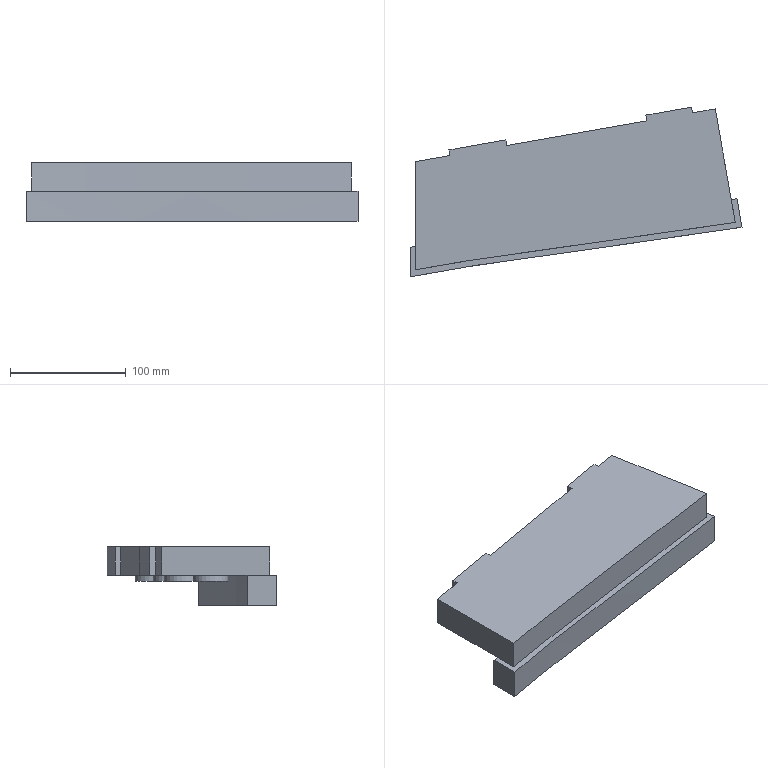Part | NX | features solid 2 | 1 solid | 30 faces | box 287.116 x 146.679 x 51 mm | volume 862735 mm3 | plane 22 | cylinder 5 | spline 3 | commonest cylinder face diameters 30 x5
STEP:
#1=CARTESIAN_POINT('',(-45.711,651.288,20.));
#2=VERTEX_POINT('',#1);
#3=CARTESIAN_POINT('',(-26.015,654.761,20.));
#4=VERTEX_POINT('',#3);
#5=CARTESIAN_POINT('',(-289.132,608.367,20.));
#6=DIRECTION('',(0.9848,0.1736,0.));
#7=VECTOR('',#6,1000.);
#8=LINE('',#5,#7);
#9=EDGE_CURVE('',#2,#4,#8,.T.);
#10=ORIENTED_EDGE('',*,*,#9,.F.);
#11=CARTESIAN_POINT('',(-45.711,651.288,45.));
#12=VERTEX_POINT('',#11);
#13=CARTESIAN_POINT('',(-45.711,651.288,51.));
#14=DIRECTION('',(0.,0.,-1.));
#15=VECTOR('',#14,1000.);
#16=LINE('',#13,#15);
#17=EDGE_CURVE('',#12,#2,#16,.T.);
#18=ORIENTED_EDGE('',*,*,#17,.F.);
#19=CARTESIAN_POINT('',(-26.015,654.761,45.));
#20=VERTEX_POINT('',#19);
#21=CARTESIAN_POINT('',(-289.132,608.367,45.));
#22=DIRECTION('',(0.9848,0.1736,0.));
#23=VECTOR('',#22,1000.);
#24=LINE('',#21,#23);
#25=EDGE_CURVE('',#12,#20,#24,.T.);
#26=ORIENTED_EDGE('',*,*,#25,.T.);
#27=CARTESIAN_POINT('',(-26.015,654.761,51.));
#28=DIRECTION('',(0.,0.,-1.));
#29=VECTOR('',#28,1000.);
#30=LINE('',#27,#29);
#31=EDGE_CURVE('',#20,#4,#30,.T.);
#32=ORIENTED_EDGE('',*,*,#31,.T.);
#33=EDGE_LOOP('',(#10,#18,#26,#32));
#34=FACE_BOUND('',#33,.T.);
#35=CARTESIAN_POINT('',(-289.132,608.367,51.));
#36=DIRECTION('',(-0.1736,0.9848,0.));
#37=DIRECTION('',(-0.9848,-0.1736,0.));
#38=AXIS2_PLACEMENT_3D('',#35,#36,#37);
#39=PLANE('',#38);
#40=ADVANCED_FACE('',(#34),#39,.T.);
#41=CARTESIAN_POINT('',(-85.103,644.343,45.));
#42=VERTEX_POINT('',#41);
#43=CARTESIAN_POINT('',(-85.103,644.343,20.));
#44=VERTEX_POINT('',#43);
#45=CARTESIAN_POINT('',(-85.103,644.343,51.));
#46=DIRECTION('',(0.,0.,-1.));
#47=VECTOR('',#46,1000.);
#48=LINE('',#45,#47);
#49=EDGE_CURVE('',#42,#44,#48,.T.);
#50=ORIENTED_EDGE('',*,*,#49,.T.);
#51=CARTESIAN_POINT('',(-206.215,622.987,20.));
#52=VERTEX_POINT('',#51);
#53=CARTESIAN_POINT('',(-289.132,608.367,20.));
#54=DIRECTION('',(0.9848,0.1736,0.));
#55=VECTOR('',#54,1000.);
#56=LINE('',#53,#55);
#57=EDGE_CURVE('',#52,#44,#56,.T.);
#58=ORIENTED_EDGE('',*,*,#57,.F.);
#59=CARTESIAN_POINT('',(-206.215,622.987,45.));
#60=VERTEX_POINT('',#59);
#61=CARTESIAN_POINT('',(-206.215,622.987,51.));
#62=DIRECTION('',(0.,0.,-1.));
#63=VECTOR('',#62,1000.);
#64=LINE('',#61,#63);
#65=EDGE_CURVE('',#60,#52,#64,.T.);
#66=ORIENTED_EDGE('',*,*,#65,.F.);
#67=CARTESIAN_POINT('',(-289.132,608.367,45.));
#68=DIRECTION('',(0.9848,0.1736,0.));
#69=VECTOR('',#68,1000.);
#70=LINE('',#67,#69);
#71=EDGE_CURVE('',#60,#42,#70,.T.);
#72=ORIENTED_EDGE('',*,*,#71,.T.);
#73=EDGE_LOOP('',(#50,#58,#66,#72));
#74=FACE_BOUND('',#73,.T.);
#75=CARTESIAN_POINT('',(-289.132,608.367,51.));
#76=DIRECTION('',(-0.1736,0.9848,0.));
#77=DIRECTION('',(-0.9848,-0.1736,0.));
#78=AXIS2_PLACEMENT_3D('',#75,#76,#77);
#79=PLANE('',#78);
#80=ADVANCED_FACE('',(#74),#79,.T.);
#81=CARTESIAN_POINT('',(-255.456,614.305,45.));
#82=VERTEX_POINT('',#81);
#83=CARTESIAN_POINT('',(-255.456,614.305,20.));
#84=VERTEX_POINT('',#83);
#85=CARTESIAN_POINT('',(-255.456,614.305,51.));
#86=DIRECTION('',(0.,0.,-1.));
#87=VECTOR('',#86,1000.);
#88=LINE('',#85,#87);
#89=EDGE_CURVE('',#82,#84,#88,.T.);
#90=ORIENTED_EDGE('',*,*,#89,.T.);
#91=CARTESIAN_POINT('',(-285.,609.095,20.));
#92=VERTEX_POINT('',#91);
#93=CARTESIAN_POINT('',(-289.132,608.367,20.));
#94=DIRECTION('',(0.9848,0.1736,0.));
#95=VECTOR('',#94,1000.);
#96=LINE('',#93,#95);
#97=EDGE_CURVE('',#92,#84,#96,.T.);
#98=ORIENTED_EDGE('',*,*,#97,.F.);
#99=CARTESIAN_POINT('',(-285.,609.095,45.));
#100=VERTEX_POINT('',#99);
#101=CARTESIAN_POINT('',(-285.,609.095,51.));
#102=DIRECTION('',(0.,0.,-1.));
#103=VECTOR('',#102,1000.);
#104=LINE('',#101,#103);
#105=EDGE_CURVE('',#100,#92,#104,.T.);
#106=ORIENTED_EDGE('',*,*,#105,.F.);
#107=CARTESIAN_POINT('',(-289.132,608.367,45.));
#108=DIRECTION('',(0.9848,0.1736,0.));
#109=VECTOR('',#108,1000.);
#110=LINE('',#107,#109);
#111=EDGE_CURVE('',#100,#82,#110,.T.);
#112=ORIENTED_EDGE('',*,*,#111,.T.);
#113=EDGE_LOOP('',(#90,#98,#106,#112));
#114=FACE_BOUND('',#113,.T.);
#115=CARTESIAN_POINT('',(-289.132,608.367,51.));
#116=DIRECTION('',(-0.1736,0.9848,0.));
#117=DIRECTION('',(-0.9848,-0.1736,0.));
#118=AXIS2_PLACEMENT_3D('',#115,#116,#117);
#119=PLANE('',#118);
#120=ADVANCED_FACE('',(#114),#119,.T.);
#121=CARTESIAN_POINT('',(-290.,535.006,20.));
#122=VERTEX_POINT('',#121);
#123=CARTESIAN_POINT('',(-290.,509.533,20.));
#124=VERTEX_POINT('',#123);
#125=CARTESIAN_POINT('',(-290.,509.533,20.));
#126=DIRECTION('',(0.,-1.,0.));
#127=VECTOR('',#126,1000.);
#128=LINE('',#125,#127);
#129=EDGE_CURVE('',#122,#124,#128,.T.);
#130=ORIENTED_EDGE('',*,*,#129,.F.);
#131=CARTESIAN_POINT('',(-290.,535.006,-6.));
#132=VERTEX_POINT('',#131);
#133=CARTESIAN_POINT('',(-290.,535.006,45.));
#134=DIRECTION('',(0.,0.,-1.));
#135=VECTOR('',#134,1000.);
#136=LINE('',#133,#135);
#137=EDGE_CURVE('',#122,#132,#136,.T.);
#138=ORIENTED_EDGE('',*,*,#137,.T.);
#139=CARTESIAN_POINT('',(-290.,509.533,-6.));
#140=VERTEX_POINT('',#139);
#141=CARTESIAN_POINT('',(-290.,509.533,-6.));
#142=DIRECTION('',(0.,1.,0.));
#143=VECTOR('',#142,1000.);
#144=LINE('',#141,#143);
#145=EDGE_CURVE('',#140,#132,#144,.T.);
#146=ORIENTED_EDGE('',*,*,#145,.F.);
#147=CARTESIAN_POINT('',(-290.,509.533,45.));
#148=DIRECTION('',(0.,0.,-1.));
#149=VECTOR('',#148,1000.);
#150=LINE('',#147,#149);
#151=EDGE_CURVE('',#124,#140,#150,.T.);
#152=ORIENTED_EDGE('',*,*,#151,.F.);
#153=EDGE_LOOP('',(#130,#138,#146,#152));
#154=FACE_BOUND('',#153,.T.);
#155=CARTESIAN_POINT('',(-290.,535.006,51.));
#156=DIRECTION('',(-1.,0.,0.));
#157=DIRECTION('',(0.,0.,1.));
#158=AXIS2_PLACEMENT_3D('',#155,#156,#157);
#159=PLANE('',#158);
#160=ADVANCED_FACE('',(#154),#159,.T.);
#161=CARTESIAN_POINT('',(-7.231,577.029,20.));
#162=VERTEX_POINT('',#161);
#163=CARTESIAN_POINT('',(-7.231,577.029,-6.));
#164=VERTEX_POINT('',#163);
#165=CARTESIAN_POINT('',(-7.231,577.029,45.));
#166=DIRECTION('',(0.,0.,-1.));
#167=VECTOR('',#166,1000.);
#168=LINE('',#165,#167);
#169=EDGE_CURVE('',#162,#164,#168,.T.);
#170=ORIENTED_EDGE('',*,*,#169,.F.);
#171=CARTESIAN_POINT('',(-2.884,552.378,20.));
#172=VERTEX_POINT('',#171);
#173=CARTESIAN_POINT('',(-2.884,552.378,20.));
#174=DIRECTION('',(0.1736,-0.9848,0.));
#175=VECTOR('',#174,1000.);
#176=LINE('',#173,#175);
#177=EDGE_CURVE('',#162,#172,#176,.T.);
#178=ORIENTED_EDGE('',*,*,#177,.T.);
#179=CARTESIAN_POINT('',(-2.884,552.378,-6.));
#180=VERTEX_POINT('',#179);
#181=CARTESIAN_POINT('',(-2.884,552.378,45.));
#182=DIRECTION('',(0.,0.,-1.));
#183=VECTOR('',#182,1000.);
#184=LINE('',#181,#183);
#185=EDGE_CURVE('',#172,#180,#184,.T.);
#186=ORIENTED_EDGE('',*,*,#185,.T.);
#187=CARTESIAN_POINT('',(-2.884,552.378,-6.));
#188=DIRECTION('',(-0.1736,0.9848,0.));
#189=VECTOR('',#188,1000.);
#190=LINE('',#187,#189);
#191=EDGE_CURVE('',#180,#164,#190,.T.);
#192=ORIENTED_EDGE('',*,*,#191,.T.);
#193=EDGE_LOOP('',(#170,#178,#186,#192));
#194=FACE_BOUND('',#193,.T.);
#195=CARTESIAN_POINT('',(-7.231,577.029,51.));
#196=DIRECTION('',(-0.9848,-0.1736,0.));
#197=DIRECTION('',(0.1736,-0.9848,0.));
#198=AXIS2_PLACEMENT_3D('',#195,#196,#197);
#199=PLANE('',#198);
#200=ADVANCED_FACE('',(#194),#199,.F.);
#201=CARTESIAN_POINT('',(-8.712,556.632,45.));
#202=VERTEX_POINT('',#201);
#203=CARTESIAN_POINT('',(-7.808,551.51,45.));
#204=DIRECTION('',(-0.1736,0.9848,0.));
#205=VECTOR('',#204,1000.);
#206=LINE('',#203,#205);
#207=EDGE_CURVE('',#202,#20,#206,.T.);
#208=ORIENTED_EDGE('',*,*,#207,.F.);
#209=CARTESIAN_POINT('',(-8.712,556.632,20.));
#210=VERTEX_POINT('',#209);
#211=CARTESIAN_POINT('',(-8.712,556.632,32.5));
#212=DIRECTION('',(0.,0.,1.));
#213=VECTOR('',#212,1000.);
#214=LINE('',#211,#213);
#215=EDGE_CURVE('',#202,#210,#214,.F.);
#216=ORIENTED_EDGE('',*,*,#215,.T.);
#217=CARTESIAN_POINT('',(-12.189,576.354,20.));
#218=VERTEX_POINT('',#217);
#219=CARTESIAN_POINT('',(-7.808,551.51,20.));
#220=DIRECTION('',(-0.1736,0.9848,0.));
#221=VECTOR('',#220,1000.);
#222=LINE('',#219,#221);
#223=EDGE_CURVE('',#210,#218,#222,.T.);
#224=ORIENTED_EDGE('',*,*,#223,.T.);
#225=CARTESIAN_POINT('',(-7.808,551.51,20.));
#226=DIRECTION('',(-0.1736,0.9848,0.));
#227=VECTOR('',#226,1000.);
#228=LINE('',#225,#227);
#229=EDGE_CURVE('',#218,#4,#228,.T.);
#230=ORIENTED_EDGE('',*,*,#229,.T.);
#231=ORIENTED_EDGE('',*,*,#31,.F.);
#232=EDGE_LOOP('',(#208,#216,#224,#230,#231));
#233=FACE_BOUND('',#232,.T.);
#234=CARTESIAN_POINT('',(-7.808,551.51,20.));
#235=DIRECTION('',(0.9848,0.1736,0.));
#236=DIRECTION('',(-0.1736,0.9848,0.));
#237=AXIS2_PLACEMENT_3D('',#234,#235,#236);
#238=PLANE('',#237);
#239=ADVANCED_FACE('',(#233),#238,.T.);
#240=CARTESIAN_POINT('',(-209.084,591.878,20.));
#241=VERTEX_POINT('',#240);
#242=CARTESIAN_POINT('',(-224.084,591.878,20.));
#243=DIRECTION('',(0.,0.,-1.));
#244=DIRECTION('',(1.,0.,0.));
#245=AXIS2_PLACEMENT_3D('',#242,#243,#244);
#246=CIRCLE('',#245,15.);
#247=EDGE_CURVE('',#241,#241,#246,.T.);
#248=ORIENTED_EDGE('',*,*,#247,.T.);
#249=EDGE_LOOP('',(#248));
#250=FACE_BOUND('',#249,.T.);
#251=CARTESIAN_POINT('',(-209.084,591.878,15.));
#252=VERTEX_POINT('',#251);
#253=CARTESIAN_POINT('',(-224.084,591.878,15.));
#254=DIRECTION('',(0.,0.,-1.));
#255=DIRECTION('',(1.,0.,0.));
#256=AXIS2_PLACEMENT_3D('',#253,#254,#255);
#257=CIRCLE('',#256,15.);
#258=EDGE_CURVE('',#252,#252,#257,.T.);
#259=ORIENTED_EDGE('',*,*,#258,.F.);
#260=EDGE_LOOP('',(#259));
#261=FACE_BOUND('',#260,.T.);
#262=CARTESIAN_POINT('',(-224.084,591.878,20.));
#263=DIRECTION('',(0.,0.,-1.));
#264=DIRECTION('',(-1.,0.,0.));
#265=AXIS2_PLACEMENT_3D('',#262,#263,#264);
#266=CYLINDRICAL_SURFACE('',#265,15.);
#267=ADVANCED_FACE('',(#250,#261),#266,.T.);
#268=ORIENTED_EDGE('',*,*,#258,.T.);
#269=EDGE_LOOP('',(#268));
#270=FACE_BOUND('',#269,.T.);
#271=CARTESIAN_POINT('',(-224.084,591.878,15.));
#272=DIRECTION('',(0.,0.,-1.));
#273=DIRECTION('',(-1.,0.,0.));
#274=AXIS2_PLACEMENT_3D('',#271,#272,#273);
#275=PLANE('',#274);
#276=ADVANCED_FACE('',(#270),#275,.T.);
#277=CARTESIAN_POINT('',(-129.084,601.878,20.));
#278=VERTEX_POINT('',#277);
#279=CARTESIAN_POINT('',(-144.084,601.878,20.));
#280=DIRECTION('',(0.,0.,-1.));
#281=DIRECTION('',(1.,0.,0.));
#282=AXIS2_PLACEMENT_3D('',#279,#280,#281);
#283=CIRCLE('',#282,15.);
#284=EDGE_CURVE('',#278,#278,#283,.T.);
#285=ORIENTED_EDGE('',*,*,#284,.T.);
#286=EDGE_LOOP('',(#285));
#287=FACE_BOUND('',#286,.T.);
#288=CARTESIAN_POINT('',(-129.084,601.878,15.));
#289=VERTEX_POINT('',#288);
#290=CARTESIAN_POINT('',(-144.084,601.878,15.));
#291=DIRECTION('',(0.,0.,-1.));
#292=DIRECTION('',(1.,0.,0.));
#293=AXIS2_PLACEMENT_3D('',#290,#291,#292);
#294=CIRCLE('',#293,15.);
#295=EDGE_CURVE('',#289,#289,#294,.T.);
#296=ORIENTED_EDGE('',*,*,#295,.F.);
#297=EDGE_LOOP('',(#296));
#298=FACE_BOUND('',#297,.T.);
#299=CARTESIAN_POINT('',(-144.084,601.878,20.));
#300=DIRECTION('',(0.,0.,-1.));
#301=DIRECTION('',(-1.,0.,0.));
#302=AXIS2_PLACEMENT_3D('',#299,#300,#301);
#303=CYLINDRICAL_SURFACE('',#302,15.);
#304=ADVANCED_FACE('',(#287,#298),#303,.T.);
#305=ORIENTED_EDGE('',*,*,#295,.T.);
#306=EDGE_LOOP('',(#305));
#307=FACE_BOUND('',#306,.T.);
#308=CARTESIAN_POINT('',(-144.084,601.878,15.));
#309=DIRECTION('',(0.,0.,-1.));
#310=DIRECTION('',(-1.,0.,0.));
#311=AXIS2_PLACEMENT_3D('',#308,#309,#310);
#312=PLANE('',#311);
#313=ADVANCED_FACE('',(#307),#312,.T.);
#314=CARTESIAN_POINT('',(-64.084,616.878,20.));
#315=VERTEX_POINT('',#314);
#316=CARTESIAN_POINT('',(-79.084,616.878,20.));
#317=DIRECTION('',(0.,0.,-1.));
#318=DIRECTION('',(1.,0.,0.));
#319=AXIS2_PLACEMENT_3D('',#316,#317,#318);
#320=CIRCLE('',#319,15.);
#321=EDGE_CURVE('',#315,#315,#320,.T.);
#322=ORIENTED_EDGE('',*,*,#321,.T.);
#323=EDGE_LOOP('',(#322));
#324=FACE_BOUND('',#323,.T.);
#325=CARTESIAN_POINT('',(-64.084,616.878,15.));
#326=VERTEX_POINT('',#325);
#327=CARTESIAN_POINT('',(-79.084,616.878,15.));
#328=DIRECTION('',(0.,0.,-1.));
#329=DIRECTION('',(1.,0.,0.));
#330=AXIS2_PLACEMENT_3D('',#327,#328,#329);
#331=CIRCLE('',#330,15.);
#332=EDGE_CURVE('',#326,#326,#331,.T.);
#333=ORIENTED_EDGE('',*,*,#332,.F.);
#334=EDGE_LOOP('',(#333));
#335=FACE_BOUND('',#334,.T.);
#336=CARTESIAN_POINT('',(-79.084,616.878,20.));
#337=DIRECTION('',(0.,0.,-1.));
#338=DIRECTION('',(-1.,0.,0.));
#339=AXIS2_PLACEMENT_3D('',#336,#337,#338);
#340=CYLINDRICAL_SURFACE('',#339,15.);
#341=ADVANCED_FACE('',(#324,#335),#340,.T.);
#342=ORIENTED_EDGE('',*,*,#332,.T.);
#343=EDGE_LOOP('',(#342));
#344=FACE_BOUND('',#343,.T.);
#345=CARTESIAN_POINT('',(-79.084,616.878,15.));
#346=DIRECTION('',(0.,0.,-1.));
#347=DIRECTION('',(-1.,0.,0.));
#348=AXIS2_PLACEMENT_3D('',#345,#346,#347);
#349=PLANE('',#348);
#350=ADVANCED_FACE('',(#344),#349,.T.);
#351=CARTESIAN_POINT('',(-244.084,566.878,20.));
#352=VERTEX_POINT('',#351);
#353=CARTESIAN_POINT('',(-259.084,566.878,20.));
#354=DIRECTION('',(0.,0.,-1.));
#355=DIRECTION('',(1.,0.,0.));
#356=AXIS2_PLACEMENT_3D('',#353,#354,#355);
#357=CIRCLE('',#356,15.);
#358=EDGE_CURVE('',#352,#352,#357,.T.);
#359=ORIENTED_EDGE('',*,*,#358,.T.);
#360=EDGE_LOOP('',(#359));
#361=FACE_BOUND('',#360,.T.);
#362=CARTESIAN_POINT('',(-244.084,566.878,15.));
#363=VERTEX_POINT('',#362);
#364=CARTESIAN_POINT('',(-259.084,566.878,15.));
#365=DIRECTION('',(0.,0.,-1.));
#366=DIRECTION('',(1.,0.,0.));
#367=AXIS2_PLACEMENT_3D('',#364,#365,#366);
#368=CIRCLE('',#367,15.);
#369=EDGE_CURVE('',#363,#363,#368,.T.);
#370=ORIENTED_EDGE('',*,*,#369,.F.);
#371=EDGE_LOOP('',(#370));
#372=FACE_BOUND('',#371,.T.);
#373=CARTESIAN_POINT('',(-259.084,566.878,20.));
#374=DIRECTION('',(0.,0.,-1.));
#375=DIRECTION('',(-1.,0.,0.));
#376=AXIS2_PLACEMENT_3D('',#373,#374,#375);
#377=CYLINDRICAL_SURFACE('',#376,15.);
#378=ADVANCED_FACE('',(#361,#372),#377,.T.);
#379=ORIENTED_EDGE('',*,*,#369,.T.);
#380=EDGE_LOOP('',(#379));
#381=FACE_BOUND('',#380,.T.);
#382=CARTESIAN_POINT('',(-259.084,566.878,15.));
#383=DIRECTION('',(0.,0.,-1.));
#384=DIRECTION('',(-1.,0.,0.));
#385=AXIS2_PLACEMENT_3D('',#382,#383,#384);
#386=PLANE('',#385);
#387=ADVANCED_FACE('',(#381),#386,.T.);
#388=CARTESIAN_POINT('',(-29.084,601.878,20.));
#389=VERTEX_POINT('',#388);
#390=CARTESIAN_POINT('',(-44.084,601.878,20.));
#391=DIRECTION('',(0.,0.,-1.));
#392=DIRECTION('',(1.,0.,0.));
#393=AXIS2_PLACEMENT_3D('',#390,#391,#392);
#394=CIRCLE('',#393,15.);
#395=EDGE_CURVE('',#389,#389,#394,.T.);
#396=ORIENTED_EDGE('',*,*,#395,.T.);
#397=EDGE_LOOP('',(#396));
#398=FACE_BOUND('',#397,.T.);
#399=CARTESIAN_POINT('',(-29.084,601.878,15.));
#400=VERTEX_POINT('',#399);
#401=CARTESIAN_POINT('',(-44.084,601.878,15.));
#402=DIRECTION('',(0.,0.,-1.));
#403=DIRECTION('',(1.,0.,0.));
#404=AXIS2_PLACEMENT_3D('',#401,#402,#403);
#405=CIRCLE('',#404,15.);
#406=EDGE_CURVE('',#400,#400,#405,.T.);
#407=ORIENTED_EDGE('',*,*,#406,.F.);
#408=EDGE_LOOP('',(#407));
#409=FACE_BOUND('',#408,.T.);
#410=CARTESIAN_POINT('',(-44.084,601.878,20.));
#411=DIRECTION('',(0.,0.,-1.));
#412=DIRECTION('',(-1.,0.,0.));
#413=AXIS2_PLACEMENT_3D('',#410,#411,#412);
#414=CYLINDRICAL_SURFACE('',#413,15.);
#415=ADVANCED_FACE('',(#398,#409),#414,.T.);
#416=ORIENTED_EDGE('',*,*,#406,.T.);
#417=EDGE_LOOP('',(#416));
#418=FACE_BOUND('',#417,.T.);
#419=CARTESIAN_POINT('',(-44.084,601.878,15.));
#420=DIRECTION('',(0.,0.,-1.));
#421=DIRECTION('',(-1.,0.,0.));
#422=AXIS2_PLACEMENT_3D('',#419,#420,#421);
#423=PLANE('',#422);
#424=ADVANCED_FACE('',(#418),#423,.T.);
#425=ORIENTED_EDGE('',*,*,#65,.T.);
#426=CARTESIAN_POINT('',(-207.084,627.911,20.));
#427=VERTEX_POINT('',#426);
#428=CARTESIAN_POINT('',(-193.101,548.61,20.));
#429=DIRECTION('',(0.1736,-0.9848,0.));
#430=VECTOR('',#429,1000.);
#431=LINE('',#428,#430);
#432=EDGE_CURVE('',#427,#52,#431,.T.);
#433=ORIENTED_EDGE('',*,*,#432,.F.);
#434=CARTESIAN_POINT('',(-207.084,627.911,45.));
#435=VERTEX_POINT('',#434);
#436=CARTESIAN_POINT('',(-207.084,627.911,51.));
#437=DIRECTION('',(0.,0.,-1.));
#438=VECTOR('',#437,1000.);
#439=LINE('',#436,#438);
#440=EDGE_CURVE('',#435,#427,#439,.T.);
#441=ORIENTED_EDGE('',*,*,#440,.F.);
#442=CARTESIAN_POINT('',(-193.101,548.61,45.));
#443=DIRECTION('',(0.1736,-0.9848,0.));
#444=VECTOR('',#443,1000.);
#445=LINE('',#442,#444);
#446=EDGE_CURVE('',#435,#60,#445,.T.);
#447=ORIENTED_EDGE('',*,*,#446,.T.);
#448=EDGE_LOOP('',(#425,#433,#441,#447));
#449=FACE_BOUND('',#448,.T.);
#450=CARTESIAN_POINT('',(-207.084,627.911,51.));
#451=DIRECTION('',(-0.9848,-0.1736,0.));
#452=DIRECTION('',(0.1736,-0.9848,0.));
#453=AXIS2_PLACEMENT_3D('',#450,#451,#452);
#454=PLANE('',#453);
#455=ADVANCED_FACE('',(#449),#454,.F.);
#456=ORIENTED_EDGE('',*,*,#89,.F.);
#457=CARTESIAN_POINT('',(-256.324,619.229,45.));
#458=VERTEX_POINT('',#457);
#459=CARTESIAN_POINT('',(-256.324,619.229,45.));
#460=DIRECTION('',(0.1736,-0.9848,0.));
#461=VECTOR('',#460,1000.);
#462=LINE('',#459,#461);
#463=EDGE_CURVE('',#458,#82,#462,.T.);
#464=ORIENTED_EDGE('',*,*,#463,.F.);
#465=CARTESIAN_POINT('',(-256.324,619.229,20.));
#466=VERTEX_POINT('',#465);
#467=CARTESIAN_POINT('',(-256.324,619.229,51.));
#468=DIRECTION('',(0.,0.,-1.));
#469=VECTOR('',#468,1000.);
#470=LINE('',#467,#469);
#471=EDGE_CURVE('',#458,#466,#470,.T.);
#472=ORIENTED_EDGE('',*,*,#471,.T.);
#473=CARTESIAN_POINT('',(-256.324,619.229,20.));
#474=DIRECTION('',(0.1736,-0.9848,0.));
#475=VECTOR('',#474,1000.);
#476=LINE('',#473,#475);
#477=EDGE_CURVE('',#466,#84,#476,.T.);
#478=ORIENTED_EDGE('',*,*,#477,.T.);
#479=EDGE_LOOP('',(#456,#464,#472,#478));
#480=FACE_BOUND('',#479,.T.);
#481=CARTESIAN_POINT('',(-256.324,619.229,51.));
#482=DIRECTION('',(-0.9848,-0.1736,0.));
#483=DIRECTION('',(0.1736,-0.9848,0.));
#484=AXIS2_PLACEMENT_3D('',#481,#482,#483);
#485=PLANE('',#484);
#486=ADVANCED_FACE('',(#480),#485,.T.);
#487=CARTESIAN_POINT('',(-290.,613.291,45.));
#488=DIRECTION('',(0.9848,0.1736,0.));
#489=VECTOR('',#488,1000.);
#490=LINE('',#487,#489);
#491=EDGE_CURVE('',#458,#435,#490,.T.);
#492=ORIENTED_EDGE('',*,*,#491,.T.);
#493=ORIENTED_EDGE('',*,*,#440,.T.);
#494=CARTESIAN_POINT('',(-290.,613.291,20.));
#495=DIRECTION('',(0.9848,0.1736,0.));
#496=VECTOR('',#495,1000.);
#497=LINE('',#494,#496);
#498=EDGE_CURVE('',#466,#427,#497,.T.);
#499=ORIENTED_EDGE('',*,*,#498,.F.);
#500=ORIENTED_EDGE('',*,*,#471,.F.);
#501=EDGE_LOOP('',(#492,#493,#499,#500));
#502=FACE_BOUND('',#501,.T.);
#503=CARTESIAN_POINT('',(-290.,613.291,51.));
#504=DIRECTION('',(-0.1736,0.9848,0.));
#505=DIRECTION('',(-0.9848,-0.1736,0.));
#506=AXIS2_PLACEMENT_3D('',#503,#504,#505);
#507=PLANE('',#506);
#508=ADVANCED_FACE('',(#502),#507,.T.);
#509=ORIENTED_EDGE('',*,*,#17,.T.);
#510=CARTESIAN_POINT('',(-46.579,656.212,20.));
#511=VERTEX_POINT('',#510);
#512=CARTESIAN_POINT('',(-46.579,656.212,20.));
#513=DIRECTION('',(0.1736,-0.9848,0.));
#514=VECTOR('',#513,1000.);
#515=LINE('',#512,#514);
#516=EDGE_CURVE('',#511,#2,#515,.T.);
#517=ORIENTED_EDGE('',*,*,#516,.F.);
#518=CARTESIAN_POINT('',(-46.579,656.212,45.));
#519=VERTEX_POINT('',#518);
#520=CARTESIAN_POINT('',(-46.579,656.212,51.));
#521=DIRECTION('',(0.,0.,-1.));
#522=VECTOR('',#521,1000.);
#523=LINE('',#520,#522);
#524=EDGE_CURVE('',#519,#511,#523,.T.);
#525=ORIENTED_EDGE('',*,*,#524,.F.);
#526=CARTESIAN_POINT('',(-46.579,656.212,45.));
#527=DIRECTION('',(0.1736,-0.9848,0.));
#528=VECTOR('',#527,1000.);
#529=LINE('',#526,#528);
#530=EDGE_CURVE('',#519,#12,#529,.T.);
#531=ORIENTED_EDGE('',*,*,#530,.T.);
#532=EDGE_LOOP('',(#509,#517,#525,#531));
#533=FACE_BOUND('',#532,.T.);
#534=CARTESIAN_POINT('',(-46.579,656.212,51.));
#535=DIRECTION('',(-0.9848,-0.1736,0.));
#536=DIRECTION('',(0.1736,-0.9848,0.));
#537=AXIS2_PLACEMENT_3D('',#534,#535,#536);
#538=PLANE('',#537);
#539=ADVANCED_FACE('',(#533),#538,.F.);
#540=ORIENTED_EDGE('',*,*,#49,.F.);
#541=CARTESIAN_POINT('',(-85.971,649.267,45.));
#542=VERTEX_POINT('',#541);
#543=CARTESIAN_POINT('',(-85.971,649.267,45.));
#544=DIRECTION('',(0.1736,-0.9848,0.));
#545=VECTOR('',#544,1000.);
#546=LINE('',#543,#545);
#547=EDGE_CURVE('',#542,#42,#546,.T.);
#548=ORIENTED_EDGE('',*,*,#547,.F.);
#549=CARTESIAN_POINT('',(-85.971,649.267,20.));
#550=VERTEX_POINT('',#549);
#551=CARTESIAN_POINT('',(-85.971,649.267,51.));
#552=DIRECTION('',(0.,0.,-1.));
#553=VECTOR('',#552,1000.);
#554=LINE('',#551,#553);
#555=EDGE_CURVE('',#542,#550,#554,.T.);
#556=ORIENTED_EDGE('',*,*,#555,.T.);
#557=CARTESIAN_POINT('',(-85.971,649.267,20.));
#558=DIRECTION('',(0.1736,-0.9848,0.));
#559=VECTOR('',#558,1000.);
#560=LINE('',#557,#559);
#561=EDGE_CURVE('',#550,#44,#560,.T.);
#562=ORIENTED_EDGE('',*,*,#561,.T.);
#563=EDGE_LOOP('',(#540,#548,#556,#562));
#564=FACE_BOUND('',#563,.T.);
#565=CARTESIAN_POINT('',(-85.971,649.267,51.));
#566=DIRECTION('',(-0.9848,-0.1736,0.));
#567=DIRECTION('',(0.1736,-0.9848,0.));
#568=AXIS2_PLACEMENT_3D('',#565,#566,#567);
#569=PLANE('',#568);
#570=ADVANCED_FACE('',(#564),#569,.T.);
#571=CARTESIAN_POINT('',(-99.951,646.802,45.));
#572=DIRECTION('',(0.9848,0.1736,0.));
#573=VECTOR('',#572,1000.);
#574=LINE('',#571,#573);
#575=EDGE_CURVE('',#542,#519,#574,.T.);
#576=ORIENTED_EDGE('',*,*,#575,.T.);
#577=ORIENTED_EDGE('',*,*,#524,.T.);
#578=CARTESIAN_POINT('',(-99.951,646.802,20.));
#579=DIRECTION('',(0.9848,0.1736,0.));
#580=VECTOR('',#579,1000.);
#581=LINE('',#578,#580);
#582=EDGE_CURVE('',#550,#511,#581,.T.);
#583=ORIENTED_EDGE('',*,*,#582,.F.);
#584=ORIENTED_EDGE('',*,*,#555,.F.);
#585=EDGE_LOOP('',(#576,#577,#583,#584));
#586=FACE_BOUND('',#585,.T.);
#587=CARTESIAN_POINT('',(-99.951,646.802,51.));
#588=DIRECTION('',(-0.1736,0.9848,0.));
#589=DIRECTION('',(-0.9848,-0.1736,0.));
#590=AXIS2_PLACEMENT_3D('',#587,#588,#589);
#591=PLANE('',#590);
#592=ADVANCED_FACE('',(#586),#591,.T.);
#593=ORIENTED_EDGE('',*,*,#223,.F.);
#594=CARTESIAN_POINT('',(-285.,515.602,20.));
#595=VERTEX_POINT('',#594);
#596=CARTESIAN_POINT('',(-8.712,556.632,20.));
#597=CARTESIAN_POINT('',(-20.246,555.065,20.));
#598=CARTESIAN_POINT('',(-43.308,551.889,20.));
#599=CARTESIAN_POINT('',(-89.36,545.049,20.));
#600=CARTESIAN_POINT('',(-146.889,536.239,20.));
#601=CARTESIAN_POINT('',(-216.16,527.295,20.));
#602=CARTESIAN_POINT('',(-262.14,519.99,20.));
#603=CARTESIAN_POINT('',(-285.,515.602,20.));
#604=B_SPLINE_CURVE_WITH_KNOTS('',3,(#596,#597,#598,#599,#600,#601,#602,#603),.UNSPECIFIED.,.F.,.F.,(4,1,1,1,1,4),(1.22,1.255,1.29,1.36,1.43,1.5),.UNSPECIFIED.);
#605=EDGE_CURVE('',#210,#595,#604,.T.);
#606=ORIENTED_EDGE('',*,*,#605,.T.);
#607=CARTESIAN_POINT('',(-285.,535.96,20.));
#608=VERTEX_POINT('',#607);
#609=CARTESIAN_POINT('',(-285.,482.459,20.));
#610=DIRECTION('',(0.,-1.,0.));
#611=VECTOR('',#610,1000.);
#612=LINE('',#609,#611);
#613=EDGE_CURVE('',#595,#608,#612,.F.);
#614=ORIENTED_EDGE('',*,*,#613,.T.);
#615=CARTESIAN_POINT('',(-290.,535.006,20.));
#616=CARTESIAN_POINT('',(-288.334,535.328,20.));
#617=CARTESIAN_POINT('',(-286.667,535.646,20.));
#618=CARTESIAN_POINT('',(-285.,535.96,20.));
#619=B_SPLINE_CURVE_WITH_KNOTS('',3,(#615,#616,#617,#618),.UNSPECIFIED.,.F.,.F.,(4,4),(1.165,1.171),.UNSPECIFIED.);
#620=EDGE_CURVE('',#122,#608,#619,.T.);
#621=ORIENTED_EDGE('',*,*,#620,.F.);
#622=ORIENTED_EDGE('',*,*,#129,.T.);
#623=CARTESIAN_POINT('',(-290.,509.533,20.));
#624=CARTESIAN_POINT('',(-266.261,514.23,20.));
#625=CARTESIAN_POINT('',(-218.498,521.957,20.));
#626=CARTESIAN_POINT('',(-146.499,531.225,20.));
#627=CARTESIAN_POINT('',(-86.712,540.4,20.));
#628=CARTESIAN_POINT('',(-38.845,547.485,20.));
#629=CARTESIAN_POINT('',(-14.872,550.749,20.));
#630=CARTESIAN_POINT('',(-2.884,552.378,20.));
#631=B_SPLINE_CURVE_WITH_KNOTS('',3,(#623,#624,#625,#626,#627,#628,#629,#630),.UNSPECIFIED.,.F.,.F.,(4,1,1,1,1,4),(0.,0.07257,0.1451,0.2177,0.254,0.2903),.UNSPECIFIED.);
#632=EDGE_CURVE('',#124,#172,#631,.T.);
#633=ORIENTED_EDGE('',*,*,#632,.T.);
#634=ORIENTED_EDGE('',*,*,#177,.F.);
#635=CARTESIAN_POINT('',(-290.,535.006,20.));
#636=CARTESIAN_POINT('',(-281.751,536.6,20.));
#637=CARTESIAN_POINT('',(-253.964,541.638,20.));
#638=CARTESIAN_POINT('',(-206.735,548.663,20.));
#639=CARTESIAN_POINT('',(-129.935,558.726,20.));
#640=CARTESIAN_POINT('',(-63.411,569.391,20.));
#641=CARTESIAN_POINT('',(-16.03,575.833,20.));
#642=CARTESIAN_POINT('',(-7.231,577.029,20.));
#643=B_SPLINE_CURVE_WITH_KNOTS('',3,(#635,#636,#637,#638,#639,#640,#641,#642),.UNSPECIFIED.,.F.,.F.,(4,1,1,1,1,4),(0.,0.0865,0.2915,0.4964,0.9063,1.),.UNSPECIFIED.);
#644=EDGE_CURVE('',#218,#162,#643,.T.);
#645=ORIENTED_EDGE('',*,*,#644,.F.);
#646=EDGE_LOOP('',(#593,#606,#614,#621,#622,#633,#634,#645));
#647=FACE_BOUND('',#646,.T.);
#648=CARTESIAN_POINT('',(-561.977,359.461,20.));
#649=DIRECTION('',(0.,0.,1.));
#650=DIRECTION('',(1.,0.,0.));
#651=AXIS2_PLACEMENT_3D('',#648,#649,#650);
#652=PLANE('',#651);
#653=ADVANCED_FACE('',(#647),#652,.T.);
#654=ORIENTED_EDGE('',*,*,#321,.F.);
#655=EDGE_LOOP('',(#654));
#656=FACE_BOUND('',#655,.T.);
#657=ORIENTED_EDGE('',*,*,#229,.F.);
#658=CARTESIAN_POINT('',(-285.,535.96,20.));
#659=CARTESIAN_POINT('',(-262.413,540.217,20.));
#660=CARTESIAN_POINT('',(-217.003,547.35,20.));
#661=CARTESIAN_POINT('',(-148.613,556.213,20.));
#662=CARTESIAN_POINT('',(-91.807,564.865,20.));
#663=CARTESIAN_POINT('',(-46.342,571.649,20.));
#664=CARTESIAN_POINT('',(-23.576,574.805,20.));
#665=CARTESIAN_POINT('',(-12.189,576.354,20.));
#666=B_SPLINE_CURVE_WITH_KNOTS('',3,(#658,#659,#660,#661,#662,#663,#664,#665),.UNSPECIFIED.,.F.,.F.,(4,1,1,1,1,4),(1.171,1.24,1.308,1.377,1.412,1.446),.UNSPECIFIED.);
#667=EDGE_CURVE('',#608,#218,#666,.T.);
#668=ORIENTED_EDGE('',*,*,#667,.F.);
#669=CARTESIAN_POINT('',(-285.,482.459,20.));
#670=DIRECTION('',(0.,-1.,0.));
#671=VECTOR('',#670,1000.);
#672=LINE('',#669,#671);
#673=EDGE_CURVE('',#608,#92,#672,.F.);
#674=ORIENTED_EDGE('',*,*,#673,.T.);
#675=ORIENTED_EDGE('',*,*,#97,.T.);
#676=ORIENTED_EDGE('',*,*,#477,.F.);
#677=ORIENTED_EDGE('',*,*,#498,.T.);
#678=ORIENTED_EDGE('',*,*,#432,.T.);
#679=ORIENTED_EDGE('',*,*,#57,.T.);
#680=ORIENTED_EDGE('',*,*,#561,.F.);
#681=ORIENTED_EDGE('',*,*,#582,.T.);
#682=ORIENTED_EDGE('',*,*,#516,.T.);
#683=ORIENTED_EDGE('',*,*,#9,.T.);
#684=EDGE_LOOP('',(#657,#668,#674,#675,#676,#677,#678,#679,#680,#681,#682,#683));
#685=FACE_BOUND('',#684,.T.);
#686=ORIENTED_EDGE('',*,*,#247,.F.);
#687=EDGE_LOOP('',(#686));
#688=FACE_BOUND('',#687,.T.);
#689=ORIENTED_EDGE('',*,*,#358,.F.);
#690=EDGE_LOOP('',(#689));
#691=FACE_BOUND('',#690,.T.);
#692=ORIENTED_EDGE('',*,*,#284,.F.);
#693=EDGE_LOOP('',(#692));
#694=FACE_BOUND('',#693,.T.);
#695=ORIENTED_EDGE('',*,*,#395,.F.);
#696=EDGE_LOOP('',(#695));
#697=FACE_BOUND('',#696,.T.);
#698=CARTESIAN_POINT('',(-561.977,359.461,20.));
#699=DIRECTION('',(0.,0.,-1.));
#700=DIRECTION('',(-1.,0.,0.));
#701=AXIS2_PLACEMENT_3D('',#698,#699,#700);
#702=PLANE('',#701);
#703=ADVANCED_FACE('',(#656,#685,#688,#691,#694,#697),#702,.T.);
#704=CARTESIAN_POINT('',(-285.,515.602,45.));
#705=VERTEX_POINT('',#704);
#706=CARTESIAN_POINT('',(-8.712,556.632,45.));
#707=CARTESIAN_POINT('',(-20.235,555.067,45.));
#708=CARTESIAN_POINT('',(-43.313,551.888,45.));
#709=CARTESIAN_POINT('',(-89.364,545.048,45.));
#710=CARTESIAN_POINT('',(-146.76,536.257,45.));
#711=CARTESIAN_POINT('',(-215.93,527.326,45.));
#712=CARTESIAN_POINT('',(-262.048,520.008,45.));
#713=CARTESIAN_POINT('',(-285.,515.602,45.));
#714=B_SPLINE_CURVE_WITH_KNOTS('',3,(#706,#707,#708,#709,#710,#711,#712,#713),.UNSPECIFIED.,.F.,.F.,(4,1,1,1,1,4),(0.01792,0.1381,0.2582,0.4985,0.7388,0.9792),.UNSPECIFIED.);
#715=EDGE_CURVE('',#202,#705,#714,.T.);
#716=ORIENTED_EDGE('',*,*,#715,.F.);
#717=ORIENTED_EDGE('',*,*,#207,.T.);
#718=ORIENTED_EDGE('',*,*,#25,.F.);
#719=ORIENTED_EDGE('',*,*,#530,.F.);
#720=ORIENTED_EDGE('',*,*,#575,.F.);
#721=ORIENTED_EDGE('',*,*,#547,.T.);
#722=ORIENTED_EDGE('',*,*,#71,.F.);
#723=ORIENTED_EDGE('',*,*,#446,.F.);
#724=ORIENTED_EDGE('',*,*,#491,.F.);
#725=ORIENTED_EDGE('',*,*,#463,.T.);
#726=ORIENTED_EDGE('',*,*,#111,.F.);
#727=CARTESIAN_POINT('',(-285.,-794.984,45.));
#728=DIRECTION('',(0.,1.,0.));
#729=VECTOR('',#728,1000.);
#730=LINE('',#727,#729);
#731=EDGE_CURVE('',#705,#100,#730,.T.);
#732=ORIENTED_EDGE('',*,*,#731,.F.);
#733=EDGE_LOOP('',(#716,#717,#718,#719,#720,#721,#722,#723,#724,#725,#726,#732));
#734=FACE_BOUND('',#733,.T.);
#735=CARTESIAN_POINT('',(-80.139,-794.984,45.));
#736=DIRECTION('',(0.,0.,1.));
#737=DIRECTION('',(1.,0.,0.));
#738=AXIS2_PLACEMENT_3D('',#735,#736,#737);
#739=PLANE('',#738);
#740=ADVANCED_FACE('',(#734),#739,.T.);
#741=ORIENTED_EDGE('',*,*,#613,.F.);
#742=CARTESIAN_POINT('',(-285.,515.602,32.5));
#743=DIRECTION('',(0.,0.,1.));
#744=VECTOR('',#743,1000.);
#745=LINE('',#742,#744);
#746=EDGE_CURVE('',#705,#595,#745,.F.);
#747=ORIENTED_EDGE('',*,*,#746,.F.);
#748=ORIENTED_EDGE('',*,*,#731,.T.);
#749=ORIENTED_EDGE('',*,*,#105,.T.);
#750=ORIENTED_EDGE('',*,*,#673,.F.);
#751=EDGE_LOOP('',(#741,#747,#748,#749,#750));
#752=FACE_BOUND('',#751,.T.);
#753=CARTESIAN_POINT('',(-285.,482.459,20.));
#754=DIRECTION('',(1.,0.,0.));
#755=DIRECTION('',(0.,0.,-1.));
#756=AXIS2_PLACEMENT_3D('',#753,#754,#755);
#757=PLANE('',#756);
#758=ADVANCED_FACE('',(#752),#757,.F.);
#759=CARTESIAN_POINT('',(-2.884,552.378,-6.));
#760=CARTESIAN_POINT('',(-11.988,551.141,-6.));
#761=CARTESIAN_POINT('',(-40.358,547.302,-6.));
#762=CARTESIAN_POINT('',(-87.902,540.194,-6.));
#763=CARTESIAN_POINT('',(-145.572,531.452,-6.));
#764=CARTESIAN_POINT('',(-203.407,523.885,-6.));
#765=CARTESIAN_POINT('',(-251.574,516.716,-6.));
#766=CARTESIAN_POINT('',(-280.368,511.439,-6.));
#767=CARTESIAN_POINT('',(-290.,509.533,-6.));
#768=B_SPLINE_CURVE_WITH_KNOTS('',3,(#759,#760,#761,#762,#763,#764,#765,#766,#767),.UNSPECIFIED.,.F.,.F.,(4,1,1,1,1,1,4),(0.,0.09493,0.2958,0.4968,0.6977,0.8986,1.),.UNSPECIFIED.);
#769=EDGE_CURVE('',#180,#140,#768,.T.);
#770=ORIENTED_EDGE('',*,*,#769,.T.);
#771=ORIENTED_EDGE('',*,*,#145,.T.);
#772=CARTESIAN_POINT('',(-290.,535.006,-6.));
#773=CARTESIAN_POINT('',(-281.751,536.6,-6.));
#774=CARTESIAN_POINT('',(-253.964,541.638,-6.));
#775=CARTESIAN_POINT('',(-206.735,548.663,-6.));
#776=CARTESIAN_POINT('',(-129.935,558.726,-6.));
#777=CARTESIAN_POINT('',(-63.411,569.391,-6.));
#778=CARTESIAN_POINT('',(-16.03,575.833,-6.));
#779=CARTESIAN_POINT('',(-7.231,577.029,-6.));
#780=B_SPLINE_CURVE_WITH_KNOTS('',3,(#772,#773,#774,#775,#776,#777,#778,#779),.UNSPECIFIED.,.F.,.F.,(4,1,1,1,1,4),(0.,0.0865,0.2915,0.4964,0.9063,1.),.UNSPECIFIED.);
#781=EDGE_CURVE('',#132,#164,#780,.T.);
#782=ORIENTED_EDGE('',*,*,#781,.T.);
#783=ORIENTED_EDGE('',*,*,#191,.F.);
#784=EDGE_LOOP('',(#770,#771,#782,#783));
#785=FACE_BOUND('',#784,.T.);
#786=CARTESIAN_POINT('',(-80.139,-794.984,-6.));
#787=DIRECTION('',(0.,0.,1.));
#788=DIRECTION('',(1.,0.,0.));
#789=AXIS2_PLACEMENT_3D('',#786,#787,#788);
#790=PLANE('',#789);
#791=ADVANCED_FACE('',(#785),#790,.F.);
#792=ORIENTED_EDGE('',*,*,#605,.F.);
#793=ORIENTED_EDGE('',*,*,#215,.F.);
#794=ORIENTED_EDGE('',*,*,#715,.T.);
#795=ORIENTED_EDGE('',*,*,#746,.T.);
#796=EDGE_LOOP('',(#792,#793,#794,#795));
#797=FACE_BOUND('',#796,.T.);
#798=CARTESIAN_POINT('',(-8.712,556.632,20.));
#799=CARTESIAN_POINT('',(-8.712,556.632,45.));
#800=CARTESIAN_POINT('',(-20.235,555.067,20.));
#801=CARTESIAN_POINT('',(-20.235,555.067,45.));
#802=CARTESIAN_POINT('',(-43.313,551.888,20.));
#803=CARTESIAN_POINT('',(-43.313,551.888,45.));
#804=CARTESIAN_POINT('',(-89.364,545.048,20.));
#805=CARTESIAN_POINT('',(-89.364,545.048,45.));
#806=CARTESIAN_POINT('',(-146.76,536.257,20.));
#807=CARTESIAN_POINT('',(-146.76,536.257,45.));
#808=CARTESIAN_POINT('',(-215.93,527.326,20.));
#809=CARTESIAN_POINT('',(-215.93,527.326,45.));
#810=CARTESIAN_POINT('',(-262.048,520.008,20.));
#811=CARTESIAN_POINT('',(-262.048,520.008,45.));
#812=CARTESIAN_POINT('',(-285.,515.602,20.));
#813=CARTESIAN_POINT('',(-285.,515.602,45.));
#814=B_SPLINE_SURFACE_WITH_KNOTS('',3,1,((#798,#799),(#800,#801),(#802,#803),(#804,#805),(#806,#807),(#808,#809),(#810,#811),(#812,#813)),.SURF_OF_LINEAR_EXTRUSION.,.F.,.F.,.F.,(4,1,1,1,1,4),(2,2),(0.01792,0.1381,0.2582,0.4985,0.7388,0.9792),(0.,1.),.UNSPECIFIED.);
#815=ADVANCED_FACE('',(#797),#814,.F.);
#816=ORIENTED_EDGE('',*,*,#632,.F.);
#817=ORIENTED_EDGE('',*,*,#151,.T.);
#818=ORIENTED_EDGE('',*,*,#769,.F.);
#819=ORIENTED_EDGE('',*,*,#185,.F.);
#820=EDGE_LOOP('',(#816,#817,#818,#819));
#821=FACE_BOUND('',#820,.T.);
#822=CARTESIAN_POINT('',(-2.884,552.378,20.));
#823=CARTESIAN_POINT('',(-2.884,552.378,-6.));
#824=CARTESIAN_POINT('',(-14.871,550.749,20.));
#825=CARTESIAN_POINT('',(-14.871,550.749,-6.));
#826=CARTESIAN_POINT('',(-38.843,547.485,20.));
#827=CARTESIAN_POINT('',(-38.843,547.485,-6.));
#828=CARTESIAN_POINT('',(-86.706,540.401,20.));
#829=CARTESIAN_POINT('',(-86.706,540.401,-6.));
#830=CARTESIAN_POINT('',(-146.493,531.225,20.));
#831=CARTESIAN_POINT('',(-146.493,531.225,-6.));
#832=CARTESIAN_POINT('',(-218.474,521.96,20.));
#833=CARTESIAN_POINT('',(-218.474,521.96,-6.));
#834=CARTESIAN_POINT('',(-266.258,514.231,20.));
#835=CARTESIAN_POINT('',(-266.258,514.231,-6.));
#836=CARTESIAN_POINT('',(-290.,509.533,20.));
#837=CARTESIAN_POINT('',(-290.,509.533,-6.));
#838=B_SPLINE_SURFACE_WITH_KNOTS('',3,1,((#822,#823),(#824,#825),(#826,#827),(#828,#829),(#830,#831),(#832,#833),(#834,#835),(#836,#837)),.SURF_OF_LINEAR_EXTRUSION.,.F.,.F.,.F.,(4,1,1,1,1,4),(2,2),(0.,0.125,0.25,0.5,0.75,1.),(0.,1.),.UNSPECIFIED.);
#839=ADVANCED_FACE('',(#821),#838,.T.);
#840=ORIENTED_EDGE('',*,*,#620,.T.);
#841=ORIENTED_EDGE('',*,*,#667,.T.);
#842=ORIENTED_EDGE('',*,*,#644,.T.);
#843=ORIENTED_EDGE('',*,*,#169,.T.);
#844=ORIENTED_EDGE('',*,*,#781,.F.);
#845=ORIENTED_EDGE('',*,*,#137,.F.);
#846=EDGE_LOOP('',(#840,#841,#842,#843,#844,#845));
#847=FACE_BOUND('',#846,.T.);
#848=CARTESIAN_POINT('',(-290.,535.006,20.));
#849=CARTESIAN_POINT('',(-290.,535.006,-6.));
#850=CARTESIAN_POINT('',(-266.16,539.612,20.));
#851=CARTESIAN_POINT('',(-266.16,539.612,-6.));
#852=CARTESIAN_POINT('',(-218.427,547.18,20.));
#853=CARTESIAN_POINT('',(-218.427,547.18,-6.));
#854=CARTESIAN_POINT('',(-148.117,556.265,20.));
#855=CARTESIAN_POINT('',(-148.117,556.265,-6.));
#856=CARTESIAN_POINT('',(-89.482,565.225,20.));
#857=CARTESIAN_POINT('',(-89.482,565.225,-6.));
#858=CARTESIAN_POINT('',(-42.497,572.211,20.));
#859=CARTESIAN_POINT('',(-42.497,572.211,-6.));
#860=CARTESIAN_POINT('',(-18.969,575.433,20.));
#861=CARTESIAN_POINT('',(-18.969,575.433,-6.));
#862=CARTESIAN_POINT('',(-7.231,577.029,20.));
#863=CARTESIAN_POINT('',(-7.231,577.029,-6.));
#864=B_SPLINE_SURFACE_WITH_KNOTS('',3,1,((#848,#849),(#850,#851),(#852,#853),(#854,#855),(#856,#857),(#858,#859),(#860,#861),(#862,#863)),.SURF_OF_LINEAR_EXTRUSION.,.F.,.F.,.F.,(4,1,1,1,1,4),(2,2),(0.,0.25,0.5,0.75,0.875,1.),(0.,1.),.UNSPECIFIED.);
#865=ADVANCED_FACE('',(#847),#864,.T.);
#866=CLOSED_SHELL('',(#40,#80,#120,#160,#200,#239,#267,#276,#304,#313,#341,#350,#378,#387,#415,#424,#455,#486,#508,#539,#570,#592,#653,#703,#740,#758,#791,#815,#839,#865));
#867=MANIFOLD_SOLID_BREP('',#866);
#868=(LENGTH_UNIT()NAMED_UNIT(*)SI_UNIT(.MILLI.,.METRE.));
#869=UNCERTAINTY_MEASURE_WITH_UNIT(LENGTH_MEASURE(0.0508),#868,'','');
#870=(NAMED_UNIT(*)PLANE_ANGLE_UNIT()SI_UNIT($,.RADIAN.));
#871=(NAMED_UNIT(*)SI_UNIT($,.STERADIAN.)SOLID_ANGLE_UNIT());
#872=(GEOMETRIC_REPRESENTATION_CONTEXT(3)GLOBAL_UNCERTAINTY_ASSIGNED_CONTEXT((#869))GLOBAL_UNIT_ASSIGNED_CONTEXT((#868,#870,#871))REPRESENTATION_CONTEXT('',''));
#873=ADVANCED_BREP_SHAPE_REPRESENTATION('',(#867),#872);